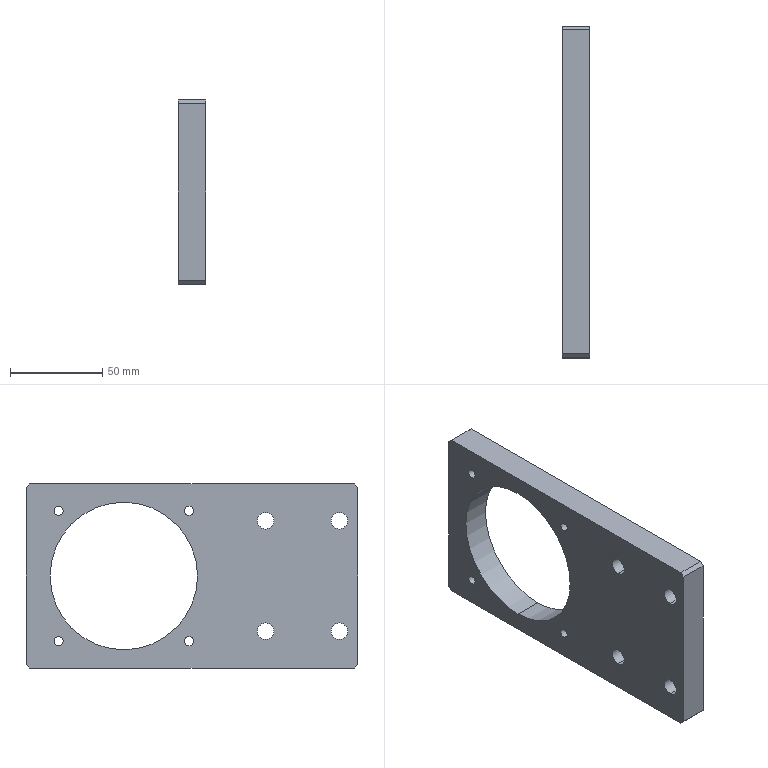Part | SolidWorks | features BaseBody 1 | 1 solid | 56 faces | box 15 x 180 x 100 mm | volume 185130 mm3 | cylinder 34 | plane 14 | cone 8 | commonest cylinder face diameters 3.3 x8 5 x8 9 x8 15 x8 80 x2